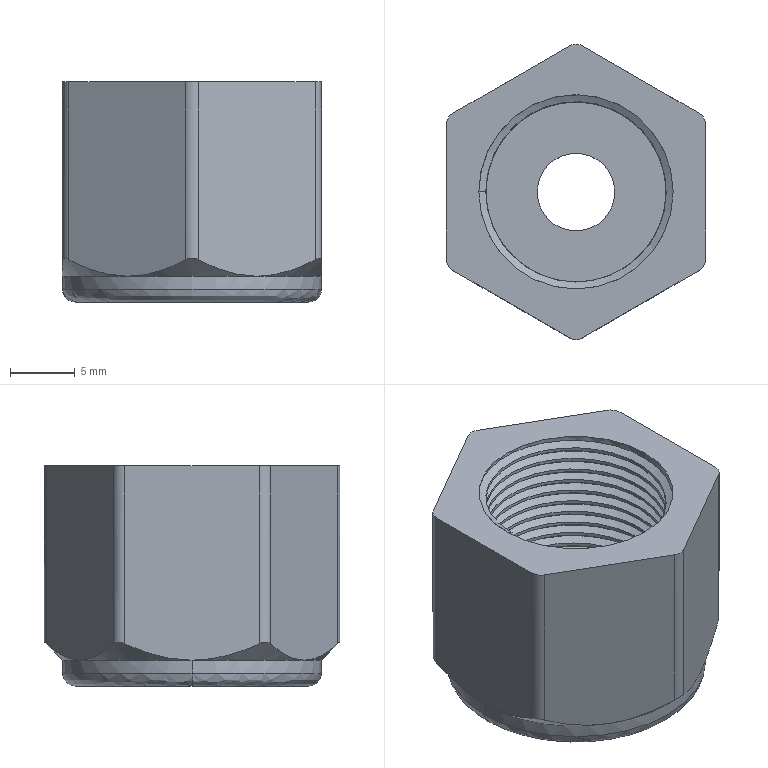Part | SolidWorks | features BaseBody 1 | 1 solid | 62 faces | box 20 x 22.785 x 17 mm | volume 3287 mm3 | cylinder 41 | plane 10 | cone 6 | spline 5 | commonest cylinder face diameters 15 x31 2 x6 6 x2 20 x2